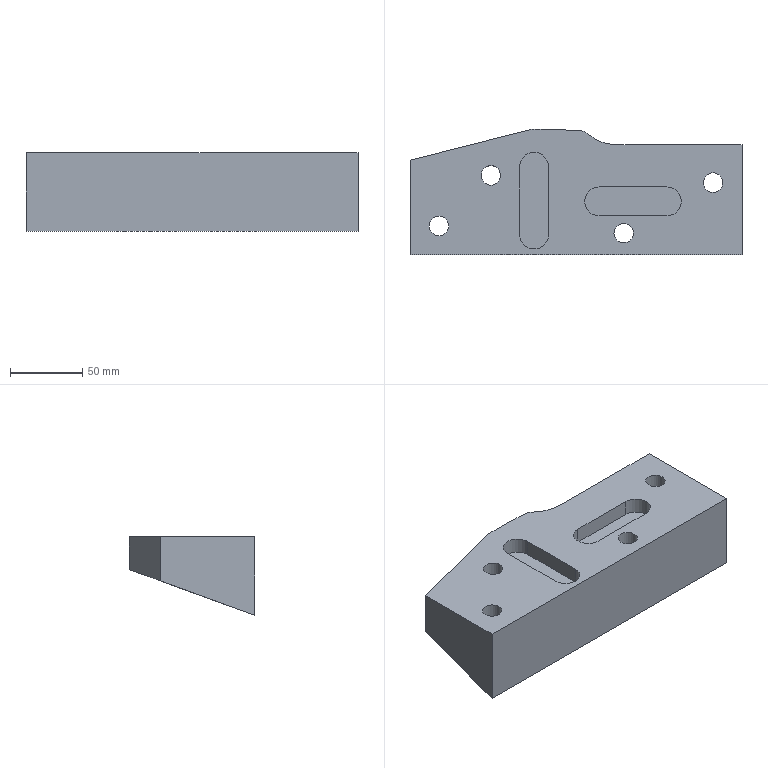Part | STEP file | lll_id3430_x_t | 1 solid | 44 faces | box 230 x 87.086 x 54.417 mm | volume 645334 mm3 | plane 20 | cylinder 18 | spline 4 | cone 2 | commonest cylinder face diameters 13.509 x4 20 x4 20.008 x4 10.505 x2 14 x2 19 x2
STEP:
#1=CARTESIAN_POINT('',(2625.,170.004,54.003));
#2=VERTEX_POINT('',#1);
#3=CARTESIAN_POINT('',(2625.,160.,50.362));
#4=DIRECTION('',(0.,-0.342,0.9397));
#5=DIRECTION('',(0.,0.9397,0.342));
#6=AXIS2_PLACEMENT_3D('',#3,#4,#5);
#7=ELLIPSE('',#6,10.646,10.004);
#8=EDGE_CURVE('',#2,#2,#7,.T.);
#9=ORIENTED_EDGE('',*,*,#8,.T.);
#10=EDGE_LOOP('',(#9));
#11=FACE_BOUND('',#10,.T.);
#12=CARTESIAN_POINT('',(2661.,205.004,66.742));
#13=VERTEX_POINT('',#12);
#14=CARTESIAN_POINT('',(2661.,195.,63.101));
#15=DIRECTION('',(0.,-0.342,0.9397));
#16=DIRECTION('',(0.,0.9397,0.342));
#17=AXIS2_PLACEMENT_3D('',#14,#15,#16);
#18=ELLIPSE('',#17,10.646,10.004);
#19=EDGE_CURVE('',#13,#13,#18,.T.);
#20=ORIENTED_EDGE('',*,*,#19,.T.);
#21=EDGE_LOOP('',(#20));
#22=FACE_BOUND('',#21,.T.);
#23=CARTESIAN_POINT('',(2650.,167.,52.91));
#24=VERTEX_POINT('',#23);
#25=CARTESIAN_POINT('',(2650.,160.,50.362));
#26=DIRECTION('',(0.,-0.342,0.9397));
#27=DIRECTION('',(0.,0.9397,0.342));
#28=AXIS2_PLACEMENT_3D('',#25,#26,#27);
#29=ELLIPSE('',#28,7.449,7.);
#30=EDGE_CURVE('',#24,#24,#29,.T.);
#31=ORIENTED_EDGE('',*,*,#30,.T.);
#32=EDGE_LOOP('',(#31));
#33=FACE_BOUND('',#32,.T.);
#34=CARTESIAN_POINT('',(2815.,200.004,64.922));
#35=VERTEX_POINT('',#34);
#36=CARTESIAN_POINT('',(2815.,190.,61.281));
#37=DIRECTION('',(0.,-0.342,0.9397));
#38=DIRECTION('',(0.,0.9397,0.342));
#39=AXIS2_PLACEMENT_3D('',#36,#37,#38);
#40=ELLIPSE('',#39,10.646,10.004);
#41=EDGE_CURVE('',#35,#35,#40,.T.);
#42=ORIENTED_EDGE('',*,*,#41,.T.);
#43=EDGE_LOOP('',(#42));
#44=FACE_BOUND('',#43,.T.);
#45=CARTESIAN_POINT('',(2753.,165.004,52.183));
#46=VERTEX_POINT('',#45);
#47=CARTESIAN_POINT('',(2753.,155.,48.542));
#48=DIRECTION('',(0.,-0.342,0.9397));
#49=DIRECTION('',(0.,0.9397,0.342));
#50=AXIS2_PLACEMENT_3D('',#47,#48,#49);
#51=ELLIPSE('',#50,10.646,10.004);
#52=EDGE_CURVE('',#46,#46,#51,.T.);
#53=ORIENTED_EDGE('',*,*,#52,.T.);
#54=EDGE_LOOP('',(#53));
#55=FACE_BOUND('',#54,.T.);
#56=CARTESIAN_POINT('',(2790.,167.,52.91));
#57=VERTEX_POINT('',#56);
#58=CARTESIAN_POINT('',(2790.,160.,50.362));
#59=DIRECTION('',(0.,-0.342,0.9397));
#60=DIRECTION('',(0.,0.9397,0.342));
#61=AXIS2_PLACEMENT_3D('',#58,#59,#60);
#62=ELLIPSE('',#61,7.449,7.);
#63=EDGE_CURVE('',#57,#57,#62,.T.);
#64=ORIENTED_EDGE('',*,*,#63,.T.);
#65=EDGE_LOOP('',(#64));
#66=FACE_BOUND('',#65,.T.);
#67=CARTESIAN_POINT('',(2835.,140.,43.083));
#68=VERTEX_POINT('',#67);
#69=CARTESIAN_POINT('',(2605.,140.,43.083));
#70=VERTEX_POINT('',#69);
#71=CARTESIAN_POINT('',(2720.,140.,43.083));
#72=DIRECTION('',(-1.,0.,0.));
#73=VECTOR('',#72,1.);
#74=LINE('',#71,#73);
#75=EDGE_CURVE('',#68,#70,#74,.T.);
#76=ORIENTED_EDGE('',*,*,#75,.T.);
#77=CARTESIAN_POINT('',(2605.,205.551,66.941));
#78=VERTEX_POINT('',#77);
#79=CARTESIAN_POINT('',(2605.,122.985,36.89));
#80=DIRECTION('',(0.,0.9397,0.342));
#81=VECTOR('',#80,1.);
#82=LINE('',#79,#81);
#83=EDGE_CURVE('',#70,#78,#82,.T.);
#84=ORIENTED_EDGE('',*,*,#83,.T.);
#85=CARTESIAN_POINT('',(2688.395,226.792,74.672));
#86=VERTEX_POINT('',#85);
#87=CARTESIAN_POINT('',(2701.697,230.18,75.905));
#88=DIRECTION('',(-0.9652,-0.2458,-0.08947));
#89=VECTOR('',#88,1.);
#90=LINE('',#87,#89);
#91=EDGE_CURVE('',#86,#78,#90,.T.);
#92=ORIENTED_EDGE('',*,*,#91,.F.);
#93=CARTESIAN_POINT('',(2691.864,227.019,74.755));
#94=VERTEX_POINT('',#93);
#95=CARTESIAN_POINT('',(2690.739,217.586,71.322));
#96=DIRECTION('',(0.,0.342,-0.9397));
#97=DIRECTION('',(0.,0.9397,0.342));
#98=AXIS2_PLACEMENT_3D('',#95,#96,#97);
#99=ELLIPSE('',#98,10.11,9.5);
#100=EDGE_CURVE('',#86,#94,#99,.T.);
#101=ORIENTED_EDGE('',*,*,#100,.T.);
#102=CARTESIAN_POINT('',(2695.813,226.8,74.675));
#103=VERTEX_POINT('',#102);
#104=CARTESIAN_POINT('',(2695.813,226.8,74.675));
#105=CARTESIAN_POINT('',(2695.461,226.798,74.675));
#106=CARTESIAN_POINT('',(2695.109,226.801,74.676));
#107=CARTESIAN_POINT('',(2694.758,226.81,74.679));
#108=CARTESIAN_POINT('',(2694.406,226.82,74.682));
#109=CARTESIAN_POINT('',(2694.054,226.834,74.688));
#110=CARTESIAN_POINT('',(2693.703,226.855,74.695));
#111=CARTESIAN_POINT('',(2693.089,226.892,74.709));
#112=CARTESIAN_POINT('',(2692.475,226.946,74.728));
#113=CARTESIAN_POINT('',(2691.864,227.019,74.755));
#114=B_SPLINE_CURVE_WITH_KNOTS('',3,(#104,#105,#106,#107,#108,#109,#110,#111,#112,#113),.UNSPECIFIED.,.F.,.F.,(4,3,3,4),(0.,0.2665,0.5331,1.),.UNSPECIFIED.);
#115=EDGE_CURVE('',#103,#94,#114,.T.);
#116=ORIENTED_EDGE('',*,*,#115,.F.);
#117=CARTESIAN_POINT('',(2704.997,226.806,74.677));
#118=VERTEX_POINT('',#117);
#119=CARTESIAN_POINT('',(2695.813,226.8,74.675));
#120=CARTESIAN_POINT('',(2696.59,226.825,74.685));
#121=CARTESIAN_POINT('',(2697.368,226.846,74.692));
#122=CARTESIAN_POINT('',(2698.146,226.859,74.697));
#123=CARTESIAN_POINT('',(2698.924,226.872,74.702));
#124=CARTESIAN_POINT('',(2699.703,226.879,74.704));
#125=CARTESIAN_POINT('',(2700.481,226.877,74.703));
#126=CARTESIAN_POINT('',(2701.986,226.873,74.702));
#127=CARTESIAN_POINT('',(2703.492,226.838,74.689));
#128=CARTESIAN_POINT('',(2704.997,226.806,74.677));
#129=B_SPLINE_CURVE_WITH_KNOTS('',3,(#119,#120,#121,#122,#123,#124,#125,#126,#127,#128),.UNSPECIFIED.,.F.,.F.,(4,3,3,4),(0.,0.2541,0.5082,1.),.UNSPECIFIED.);
#130=EDGE_CURVE('',#103,#118,#129,.T.);
#131=ORIENTED_EDGE('',*,*,#130,.T.);
#132=CARTESIAN_POINT('',(2722.606,226.048,74.402));
#133=VERTEX_POINT('',#132);
#134=CARTESIAN_POINT('',(2737.607,225.403,74.167));
#135=DIRECTION('',(-0.999,0.04298,0.01564));
#136=VECTOR('',#135,1.);
#137=LINE('',#134,#136);
#138=EDGE_CURVE('',#133,#118,#137,.T.);
#139=ORIENTED_EDGE('',*,*,#138,.F.);
#140=CARTESIAN_POINT('',(2728.715,223.469,73.463));
#141=VERTEX_POINT('',#140);
#142=CARTESIAN_POINT('',(2722.197,216.557,70.947));
#143=DIRECTION('',(0.,-0.342,0.9397));
#144=DIRECTION('',(0.,0.9397,0.342));
#145=AXIS2_PLACEMENT_3D('',#142,#143,#144);
#146=ELLIPSE('',#145,10.11,9.5);
#147=EDGE_CURVE('',#141,#133,#146,.T.);
#148=ORIENTED_EDGE('',*,*,#147,.F.);
#149=CARTESIAN_POINT('',(2744.457,216.509,70.93));
#150=VERTEX_POINT('',#149);
#151=CARTESIAN_POINT('',(2744.457,216.509,70.93));
#152=CARTESIAN_POINT('',(2738.528,217.02,71.115));
#153=CARTESIAN_POINT('',(2732.917,219.506,72.02));
#154=CARTESIAN_POINT('',(2728.715,223.469,73.463));
#155=B_SPLINE_CURVE_WITH_KNOTS('',3,(#151,#152,#153,#154),.UNSPECIFIED.,.F.,.F.,(4,4),(0.,1.),.UNSPECIFIED.);
#156=EDGE_CURVE('',#150,#141,#155,.T.);
#157=ORIENTED_EDGE('',*,*,#156,.F.);
#158=CARTESIAN_POINT('',(2753.979,216.1,70.781));
#159=VERTEX_POINT('',#158);
#160=CARTESIAN_POINT('',(2744.457,216.509,70.93));
#161=CARTESIAN_POINT('',(2745.266,216.439,70.904));
#162=CARTESIAN_POINT('',(2746.076,216.379,70.882));
#163=CARTESIAN_POINT('',(2746.887,216.327,70.863));
#164=CARTESIAN_POINT('',(2747.698,216.275,70.844));
#165=CARTESIAN_POINT('',(2748.509,216.232,70.829));
#166=CARTESIAN_POINT('',(2749.321,216.198,70.816));
#167=CARTESIAN_POINT('',(2750.873,216.133,70.793));
#168=CARTESIAN_POINT('',(2752.426,216.1,70.781));
#169=CARTESIAN_POINT('',(2753.979,216.1,70.781));
#170=B_SPLINE_CURVE_WITH_KNOTS('',3,(#160,#161,#162,#163,#164,#165,#166,#167,#168,#169),.UNSPECIFIED.,.F.,.F.,(4,3,3,4),(0.,0.2557,0.5114,1.),.UNSPECIFIED.);
#171=EDGE_CURVE('',#150,#159,#170,.T.);
#172=ORIENTED_EDGE('',*,*,#171,.T.);
#173=CARTESIAN_POINT('',(2835.,216.1,70.781));
#174=VERTEX_POINT('',#173);
#175=CARTESIAN_POINT('',(2732.617,216.1,70.781));
#176=DIRECTION('',(1.,0.,0.));
#177=VECTOR('',#176,1.);
#178=LINE('',#175,#177);
#179=EDGE_CURVE('',#159,#174,#178,.T.);
#180=ORIENTED_EDGE('',*,*,#179,.T.);
#181=CARTESIAN_POINT('',(2835.,62.167,14.754));
#182=DIRECTION('',(0.,0.9397,0.342));
#183=VECTOR('',#182,1.);
#184=LINE('',#181,#183);
#185=EDGE_CURVE('',#68,#174,#184,.T.);
#186=ORIENTED_EDGE('',*,*,#185,.F.);
#187=EDGE_LOOP('',(#76,#84,#92,#101,#116,#131,#139,#148,#157,#172,#180,#186));
#188=FACE_BOUND('',#187,.T.);
#189=CARTESIAN_POINT('',(2732.617,122.985,36.89));
#190=DIRECTION('',(0.,-0.342,0.9397));
#191=DIRECTION('',(0.,0.9397,0.342));
#192=AXIS2_PLACEMENT_3D('',#189,#190,#191);
#193=PLANE('',#192);
#194=ADVANCED_FACE('',(#11,#22,#33,#44,#55,#66,#188),#193,.F.);
#195=CARTESIAN_POINT('',(2783.,167.,97.5));
#196=VERTEX_POINT('',#195);
#197=CARTESIAN_POINT('',(2736.,167.,97.5));
#198=VERTEX_POINT('',#197);
#199=CARTESIAN_POINT('',(2685.,167.,97.5));
#200=DIRECTION('',(-1.,0.,0.));
#201=VECTOR('',#200,1.);
#202=LINE('',#199,#201);
#203=EDGE_CURVE('',#196,#198,#202,.T.);
#204=ORIENTED_EDGE('',*,*,#203,.T.);
#205=CARTESIAN_POINT('',(2736.,187.,97.5));
#206=VERTEX_POINT('',#205);
#207=CARTESIAN_POINT('',(2736.,177.,97.5));
#208=DIRECTION('',(0.,0.,-1.));
#209=DIRECTION('',(-1.,0.,0.));
#210=AXIS2_PLACEMENT_3D('',#207,#208,#209);
#211=CIRCLE('',#210,10.);
#212=EDGE_CURVE('',#198,#206,#211,.T.);
#213=ORIENTED_EDGE('',*,*,#212,.T.);
#214=CARTESIAN_POINT('',(2783.,187.,97.5));
#215=VERTEX_POINT('',#214);
#216=CARTESIAN_POINT('',(2685.,187.,97.5));
#217=DIRECTION('',(1.,0.,0.));
#218=VECTOR('',#217,1.);
#219=LINE('',#216,#218);
#220=EDGE_CURVE('',#206,#215,#219,.T.);
#221=ORIENTED_EDGE('',*,*,#220,.T.);
#222=CARTESIAN_POINT('',(2783.,177.,97.5));
#223=DIRECTION('',(0.,0.,-1.));
#224=DIRECTION('',(-1.,0.,0.));
#225=AXIS2_PLACEMENT_3D('',#222,#223,#224);
#226=CIRCLE('',#225,10.);
#227=EDGE_CURVE('',#215,#196,#226,.T.);
#228=ORIENTED_EDGE('',*,*,#227,.T.);
#229=EDGE_LOOP('',(#204,#213,#221,#228));
#230=FACE_BOUND('',#229,.T.);
#231=CARTESIAN_POINT('',(2701.,201.,97.5));
#232=VERTEX_POINT('',#231);
#233=CARTESIAN_POINT('',(2701.,154.,97.5));
#234=VERTEX_POINT('',#233);
#235=CARTESIAN_POINT('',(2701.,0.00007422,97.5));
#236=DIRECTION('',(0.,-1.,0.));
#237=VECTOR('',#236,1.);
#238=LINE('',#235,#237);
#239=EDGE_CURVE('',#232,#234,#238,.T.);
#240=ORIENTED_EDGE('',*,*,#239,.T.);
#241=CARTESIAN_POINT('',(2681.,154.,97.5));
#242=VERTEX_POINT('',#241);
#243=CARTESIAN_POINT('',(2691.,154.,97.5));
#244=DIRECTION('',(0.,0.,-1.));
#245=DIRECTION('',(-1.,0.,0.));
#246=AXIS2_PLACEMENT_3D('',#243,#244,#245);
#247=CIRCLE('',#246,10.);
#248=EDGE_CURVE('',#234,#242,#247,.T.);
#249=ORIENTED_EDGE('',*,*,#248,.T.);
#250=CARTESIAN_POINT('',(2681.,201.,97.5));
#251=VERTEX_POINT('',#250);
#252=CARTESIAN_POINT('',(2681.,0.00007422,97.5));
#253=DIRECTION('',(0.,1.,0.));
#254=VECTOR('',#253,1.);
#255=LINE('',#252,#254);
#256=EDGE_CURVE('',#242,#251,#255,.T.);
#257=ORIENTED_EDGE('',*,*,#256,.T.);
#258=CARTESIAN_POINT('',(2691.,201.,97.5));
#259=DIRECTION('',(0.,0.,-1.));
#260=DIRECTION('',(-1.,0.,0.));
#261=AXIS2_PLACEMENT_3D('',#258,#259,#260);
#262=CIRCLE('',#261,10.);
#263=EDGE_CURVE('',#251,#232,#262,.T.);
#264=ORIENTED_EDGE('',*,*,#263,.T.);
#265=EDGE_LOOP('',(#240,#249,#257,#264));
#266=FACE_BOUND('',#265,.T.);
#267=CARTESIAN_POINT('',(2618.245,160.,97.5));
#268=VERTEX_POINT('',#267);
#269=CARTESIAN_POINT('',(2625.,160.,97.5));
#270=DIRECTION('',(0.,0.,-1.));
#271=DIRECTION('',(-1.,0.,0.));
#272=AXIS2_PLACEMENT_3D('',#269,#270,#271);
#273=CIRCLE('',#272,6.755);
#274=EDGE_CURVE('',#268,#268,#273,.T.);
#275=ORIENTED_EDGE('',*,*,#274,.T.);
#276=EDGE_LOOP('',(#275));
#277=FACE_BOUND('',#276,.T.);
#278=CARTESIAN_POINT('',(2654.245,195.,97.5));
#279=VERTEX_POINT('',#278);
#280=CARTESIAN_POINT('',(2661.,195.,97.5));
#281=DIRECTION('',(0.,0.,-1.));
#282=DIRECTION('',(-1.,0.,0.));
#283=AXIS2_PLACEMENT_3D('',#280,#281,#282);
#284=CIRCLE('',#283,6.755);
#285=EDGE_CURVE('',#279,#279,#284,.T.);
#286=ORIENTED_EDGE('',*,*,#285,.T.);
#287=EDGE_LOOP('',(#286));
#288=FACE_BOUND('',#287,.T.);
#289=CARTESIAN_POINT('',(2808.245,190.,97.5));
#290=VERTEX_POINT('',#289);
#291=CARTESIAN_POINT('',(2815.,190.,97.5));
#292=DIRECTION('',(0.,0.,-1.));
#293=DIRECTION('',(-1.,0.,0.));
#294=AXIS2_PLACEMENT_3D('',#291,#292,#293);
#295=CIRCLE('',#294,6.755);
#296=EDGE_CURVE('',#290,#290,#295,.T.);
#297=ORIENTED_EDGE('',*,*,#296,.T.);
#298=EDGE_LOOP('',(#297));
#299=FACE_BOUND('',#298,.T.);
#300=CARTESIAN_POINT('',(2746.245,155.,97.5));
#301=VERTEX_POINT('',#300);
#302=CARTESIAN_POINT('',(2753.,155.,97.5));
#303=DIRECTION('',(0.,0.,-1.));
#304=DIRECTION('',(-1.,0.,0.));
#305=AXIS2_PLACEMENT_3D('',#302,#303,#304);
#306=CIRCLE('',#305,6.755);
#307=EDGE_CURVE('',#301,#301,#306,.T.);
#308=ORIENTED_EDGE('',*,*,#307,.T.);
#309=EDGE_LOOP('',(#308));
#310=FACE_BOUND('',#309,.T.);
#311=CARTESIAN_POINT('',(2835.,140.,97.5));
#312=VERTEX_POINT('',#311);
#313=CARTESIAN_POINT('',(2605.,140.,97.5));
#314=VERTEX_POINT('',#313);
#315=CARTESIAN_POINT('',(2685.,140.,97.5));
#316=DIRECTION('',(-1.,0.,0.));
#317=VECTOR('',#316,1.);
#318=LINE('',#315,#317);
#319=EDGE_CURVE('',#312,#314,#318,.T.);
#320=ORIENTED_EDGE('',*,*,#319,.F.);
#321=CARTESIAN_POINT('',(2835.,216.1,97.5));
#322=VERTEX_POINT('',#321);
#323=CARTESIAN_POINT('',(2835.,0.00007422,97.5));
#324=DIRECTION('',(0.,1.,0.));
#325=VECTOR('',#324,1.);
#326=LINE('',#323,#325);
#327=EDGE_CURVE('',#312,#322,#326,.T.);
#328=ORIENTED_EDGE('',*,*,#327,.T.);
#329=CARTESIAN_POINT('',(2753.979,216.1,97.5));
#330=VERTEX_POINT('',#329);
#331=CARTESIAN_POINT('',(2753.979,216.1,97.5));
#332=DIRECTION('',(1.,0.,0.));
#333=VECTOR('',#332,1.);
#334=LINE('',#331,#333);
#335=EDGE_CURVE('',#330,#322,#334,.T.);
#336=ORIENTED_EDGE('',*,*,#335,.F.);
#337=CARTESIAN_POINT('',(2744.457,216.509,97.5));
#338=VERTEX_POINT('',#337);
#339=CARTESIAN_POINT('',(2753.979,216.1,97.5));
#340=CARTESIAN_POINT('',(2753.166,216.1,97.5));
#341=CARTESIAN_POINT('',(2752.353,216.109,97.5));
#342=CARTESIAN_POINT('',(2751.541,216.127,97.5));
#343=CARTESIAN_POINT('',(2750.728,216.145,97.5));
#344=CARTESIAN_POINT('',(2749.916,216.171,97.5));
#345=CARTESIAN_POINT('',(2749.104,216.207,97.5));
#346=CARTESIAN_POINT('',(2747.553,216.275,97.5));
#347=CARTESIAN_POINT('',(2746.003,216.376,97.5));
#348=CARTESIAN_POINT('',(2744.457,216.509,97.5));
#349=B_SPLINE_CURVE_WITH_KNOTS('',3,(#339,#340,#341,#342,#343,#344,#345,#346,#347,#348),.UNSPECIFIED.,.F.,.F.,(4,3,3,4),(0.,0.2557,0.5115,1.),.UNSPECIFIED.);
#350=EDGE_CURVE('',#330,#338,#349,.T.);
#351=ORIENTED_EDGE('',*,*,#350,.T.);
#352=CARTESIAN_POINT('',(2728.715,223.469,97.5));
#353=VERTEX_POINT('',#352);
#354=CARTESIAN_POINT('',(2728.715,223.469,97.5));
#355=CARTESIAN_POINT('',(2732.994,219.433,97.5));
#356=CARTESIAN_POINT('',(2738.6,217.013,97.5));
#357=CARTESIAN_POINT('',(2744.457,216.509,97.5));
#358=B_SPLINE_CURVE_WITH_KNOTS('',3,(#354,#355,#356,#357),.UNSPECIFIED.,.F.,.F.,(4,4),(0.,1.),.UNSPECIFIED.);
#359=EDGE_CURVE('',#353,#338,#358,.T.);
#360=ORIENTED_EDGE('',*,*,#359,.F.);
#361=CARTESIAN_POINT('',(2722.606,226.048,97.5));
#362=VERTEX_POINT('',#361);
#363=CARTESIAN_POINT('',(2722.197,216.557,97.5));
#364=DIRECTION('',(0.,0.,1.));
#365=DIRECTION('',(-1.,0.,0.));
#366=AXIS2_PLACEMENT_3D('',#363,#364,#365);
#367=CIRCLE('',#366,9.5);
#368=EDGE_CURVE('',#353,#362,#367,.T.);
#369=ORIENTED_EDGE('',*,*,#368,.T.);
#370=CARTESIAN_POINT('',(2704.997,226.806,97.5));
#371=VERTEX_POINT('',#370);
#372=CARTESIAN_POINT('',(2694.776,227.245,97.5));
#373=DIRECTION('',(0.9991,-0.04298,0.));
#374=VECTOR('',#373,1.);
#375=LINE('',#372,#374);
#376=EDGE_CURVE('',#371,#362,#375,.T.);
#377=ORIENTED_EDGE('',*,*,#376,.F.);
#378=CARTESIAN_POINT('',(2695.813,226.8,97.5));
#379=VERTEX_POINT('',#378);
#380=CARTESIAN_POINT('',(2695.813,226.8,97.5));
#381=CARTESIAN_POINT('',(2696.59,226.825,97.5));
#382=CARTESIAN_POINT('',(2697.368,226.846,97.5));
#383=CARTESIAN_POINT('',(2698.146,226.859,97.5));
#384=CARTESIAN_POINT('',(2698.924,226.872,97.5));
#385=CARTESIAN_POINT('',(2699.703,226.879,97.5));
#386=CARTESIAN_POINT('',(2700.481,226.877,97.5));
#387=CARTESIAN_POINT('',(2701.987,226.873,97.5));
#388=CARTESIAN_POINT('',(2703.492,226.838,97.5));
#389=CARTESIAN_POINT('',(2704.997,226.806,97.5));
#390=B_SPLINE_CURVE_WITH_KNOTS('',3,(#380,#381,#382,#383,#384,#385,#386,#387,#388,#389),.UNSPECIFIED.,.F.,.F.,(4,3,3,4),(0.,0.2541,0.5082,1.),.UNSPECIFIED.);
#391=EDGE_CURVE('',#379,#371,#390,.T.);
#392=ORIENTED_EDGE('',*,*,#391,.F.);
#393=CARTESIAN_POINT('',(2691.864,227.019,97.5));
#394=VERTEX_POINT('',#393);
#395=CARTESIAN_POINT('',(2695.813,226.8,97.5));
#396=CARTESIAN_POINT('',(2695.461,226.798,97.5));
#397=CARTESIAN_POINT('',(2695.109,226.801,97.5));
#398=CARTESIAN_POINT('',(2694.758,226.81,97.5));
#399=CARTESIAN_POINT('',(2694.406,226.82,97.5));
#400=CARTESIAN_POINT('',(2694.054,226.834,97.5));
#401=CARTESIAN_POINT('',(2693.703,226.855,97.5));
#402=CARTESIAN_POINT('',(2693.089,226.892,97.5));
#403=CARTESIAN_POINT('',(2692.475,226.946,97.5));
#404=CARTESIAN_POINT('',(2691.864,227.019,97.5));
#405=B_SPLINE_CURVE_WITH_KNOTS('',3,(#395,#396,#397,#398,#399,#400,#401,#402,#403,#404),.UNSPECIFIED.,.F.,.F.,(4,3,3,4),(0.,0.2666,0.5332,1.),.UNSPECIFIED.);
#406=EDGE_CURVE('',#379,#394,#405,.T.);
#407=ORIENTED_EDGE('',*,*,#406,.T.);
#408=CARTESIAN_POINT('',(2688.395,226.792,97.5));
#409=VERTEX_POINT('',#408);
#410=CARTESIAN_POINT('',(2690.739,217.586,97.5));
#411=DIRECTION('',(0.,0.,-1.));
#412=DIRECTION('',(-1.,0.,0.));
#413=AXIS2_PLACEMENT_3D('',#410,#411,#412);
#414=CIRCLE('',#413,9.5);
#415=EDGE_CURVE('',#409,#394,#414,.T.);
#416=ORIENTED_EDGE('',*,*,#415,.F.);
#417=CARTESIAN_POINT('',(2605.,205.551,97.5));
#418=VERTEX_POINT('',#417);
#419=CARTESIAN_POINT('',(2630.962,212.164,97.5));
#420=DIRECTION('',(0.9691,0.2468,0.));
#421=VECTOR('',#420,1.);
#422=LINE('',#419,#421);
#423=EDGE_CURVE('',#418,#409,#422,.T.);
#424=ORIENTED_EDGE('',*,*,#423,.F.);
#425=CARTESIAN_POINT('',(2605.,0.,97.5));
#426=DIRECTION('',(0.,-1.,0.));
#427=VECTOR('',#426,1.);
#428=LINE('',#425,#427);
#429=EDGE_CURVE('',#418,#314,#428,.T.);
#430=ORIENTED_EDGE('',*,*,#429,.T.);
#431=EDGE_LOOP('',(#320,#328,#336,#351,#360,#369,#377,#392,#407,#416,#424,#430));
#432=FACE_BOUND('',#431,.T.);
#433=CARTESIAN_POINT('',(2685.,0.00007422,97.5));
#434=DIRECTION('',(0.,0.,-1.));
#435=DIRECTION('',(1.,0.,0.));
#436=AXIS2_PLACEMENT_3D('',#433,#434,#435);
#437=PLANE('',#436);
#438=ADVANCED_FACE('',(#230,#266,#277,#288,#299,#310,#432),#437,.F.);
#439=CARTESIAN_POINT('',(2835.,140.,652.5));
#440=DIRECTION('',(0.,0.,1.));
#441=VECTOR('',#440,1.);
#442=LINE('',#439,#441);
#443=EDGE_CURVE('',#68,#312,#442,.T.);
#444=ORIENTED_EDGE('',*,*,#443,.F.);
#445=ORIENTED_EDGE('',*,*,#185,.T.);
#446=CARTESIAN_POINT('',(2835.,216.1,652.5));
#447=DIRECTION('',(0.,0.,1.));
#448=VECTOR('',#447,1.);
#449=LINE('',#446,#448);
#450=EDGE_CURVE('',#174,#322,#449,.T.);
#451=ORIENTED_EDGE('',*,*,#450,.T.);
#452=ORIENTED_EDGE('',*,*,#327,.F.);
#453=EDGE_LOOP('',(#444,#445,#451,#452));
#454=FACE_OUTER_BOUND('',#453,.T.);
#455=CARTESIAN_POINT('',(2835.,-169.953,652.5));
#456=DIRECTION('',(-1.,0.,0.));
#457=DIRECTION('',(0.,0.,-1.));
#458=AXIS2_PLACEMENT_3D('',#455,#456,#457);
#459=PLANE('',#458);
#460=ADVANCED_FACE('',(#454),#459,.F.);
#461=ORIENTED_EDGE('',*,*,#83,.F.);
#462=CARTESIAN_POINT('',(2605.,140.,52.5));
#463=DIRECTION('',(0.,0.,-1.));
#464=VECTOR('',#463,1.);
#465=LINE('',#462,#464);
#466=EDGE_CURVE('',#314,#70,#465,.T.);
#467=ORIENTED_EDGE('',*,*,#466,.F.);
#468=ORIENTED_EDGE('',*,*,#429,.F.);
#469=CARTESIAN_POINT('',(2605.,205.551,-74.226));
#470=DIRECTION('',(0.,0.,-1.));
#471=VECTOR('',#470,1.);
#472=LINE('',#469,#471);
#473=EDGE_CURVE('',#418,#78,#472,.T.);
#474=ORIENTED_EDGE('',*,*,#473,.T.);
#475=EDGE_LOOP('',(#461,#467,#468,#474));
#476=FACE_OUTER_BOUND('',#475,.T.);
#477=CARTESIAN_POINT('',(2605.,0.,52.5));
#478=DIRECTION('',(-1.,0.,0.));
#479=DIRECTION('',(0.,0.,1.));
#480=AXIS2_PLACEMENT_3D('',#477,#478,#479);
#481=PLANE('',#480);
#482=ADVANCED_FACE('',(#476),#481,.T.);
#483=ORIENTED_EDGE('',*,*,#91,.T.);
#484=ORIENTED_EDGE('',*,*,#473,.F.);
#485=ORIENTED_EDGE('',*,*,#423,.T.);
#486=CARTESIAN_POINT('',(2688.395,226.792,-74.226));
#487=DIRECTION('',(0.,0.,-1.));
#488=VECTOR('',#487,1.);
#489=LINE('',#486,#488);
#490=EDGE_CURVE('',#409,#86,#489,.T.);
#491=ORIENTED_EDGE('',*,*,#490,.T.);
#492=EDGE_LOOP('',(#483,#484,#485,#491));
#493=FACE_OUTER_BOUND('',#492,.T.);
#494=CARTESIAN_POINT('',(2690.762,227.395,-74.226));
#495=DIRECTION('',(-0.2468,0.9691,0.));
#496=DIRECTION('',(-0.9691,-0.2468,0.));
#497=AXIS2_PLACEMENT_3D('',#494,#495,#496);
#498=PLANE('',#497);
#499=ADVANCED_FACE('',(#493),#498,.T.);
#500=ORIENTED_EDGE('',*,*,#415,.T.);
#501=CARTESIAN_POINT('',(2691.864,227.019,-74.342));
#502=DIRECTION('',(0.,0.,1.));
#503=VECTOR('',#502,1.);
#504=LINE('',#501,#503);
#505=EDGE_CURVE('',#94,#394,#504,.T.);
#506=ORIENTED_EDGE('',*,*,#505,.F.);
#507=ORIENTED_EDGE('',*,*,#100,.F.);
#508=ORIENTED_EDGE('',*,*,#490,.F.);
#509=EDGE_LOOP('',(#500,#506,#507,#508));
#510=FACE_OUTER_BOUND('',#509,.T.);
#511=CARTESIAN_POINT('',(2690.739,217.586,75.739));
#512=DIRECTION('',(0.,0.,1.));
#513=DIRECTION('',(-1.,0.,0.));
#514=AXIS2_PLACEMENT_3D('',#511,#512,#513);
#515=CYLINDRICAL_SURFACE('',#514,9.5);
#516=ADVANCED_FACE('',(#510),#515,.T.);
#517=ORIENTED_EDGE('',*,*,#406,.F.);
#518=CARTESIAN_POINT('',(2695.813,226.8,74.675));
#519=DIRECTION('',(0.,0.,1.));
#520=VECTOR('',#519,1.);
#521=LINE('',#518,#520);
#522=EDGE_CURVE('',#103,#379,#521,.T.);
#523=ORIENTED_EDGE('',*,*,#522,.F.);
#524=ORIENTED_EDGE('',*,*,#115,.T.);
#525=ORIENTED_EDGE('',*,*,#505,.T.);
#526=EDGE_LOOP('',(#517,#523,#524,#525));
#527=FACE_OUTER_BOUND('',#526,.T.);
#528=CARTESIAN_POINT('',(2695.813,226.8,74.538));
#529=CARTESIAN_POINT('',(2695.813,226.8,97.638));
#530=CARTESIAN_POINT('',(2695.509,226.798,74.538));
#531=CARTESIAN_POINT('',(2695.509,226.798,97.637));
#532=CARTESIAN_POINT('',(2695.157,226.801,74.538));
#533=CARTESIAN_POINT('',(2695.157,226.801,97.638));
#534=CARTESIAN_POINT('',(2694.498,226.816,74.544));
#535=CARTESIAN_POINT('',(2694.498,226.816,97.644));
#536=CARTESIAN_POINT('',(2693.509,226.855,74.557));
#537=CARTESIAN_POINT('',(2693.509,226.855,97.657));
#538=CARTESIAN_POINT('',(2692.521,226.941,74.585));
#539=CARTESIAN_POINT('',(2692.521,226.941,97.685));
#540=CARTESIAN_POINT('',(2691.864,227.019,74.612));
#541=CARTESIAN_POINT('',(2691.864,227.019,97.711));
#542=B_SPLINE_SURFACE_WITH_KNOTS('',3,1,((#528,#529),(#530,#531),(#532,#533),(#534,#535),(#536,#537),(#538,#539),(#540,#541)),.UNSPECIFIED.,.F.,.F.,.F.,(4,2,1,4),(2,2),(0.,0.25,0.5,1.),(0.,1.),.UNSPECIFIED.);
#543=ADVANCED_FACE('',(#527),#542,.T.);
#544=ORIENTED_EDGE('',*,*,#391,.T.);
#545=CARTESIAN_POINT('',(2704.997,226.806,74.677));
#546=DIRECTION('',(0.,0.,1.));
#547=VECTOR('',#546,1.);
#548=LINE('',#545,#547);
#549=EDGE_CURVE('',#118,#371,#548,.T.);
#550=ORIENTED_EDGE('',*,*,#549,.F.);
#551=ORIENTED_EDGE('',*,*,#130,.F.);
#552=ORIENTED_EDGE('',*,*,#522,.T.);
#553=EDGE_LOOP('',(#544,#550,#551,#552));
#554=FACE_OUTER_BOUND('',#553,.T.);
#555=CARTESIAN_POINT('',(2704.997,226.806,74.54));
#556=CARTESIAN_POINT('',(2704.997,226.806,97.639));
#557=CARTESIAN_POINT('',(2703.442,226.839,74.552));
#558=CARTESIAN_POINT('',(2703.442,226.839,97.652));
#559=CARTESIAN_POINT('',(2701.905,226.874,74.565));
#560=CARTESIAN_POINT('',(2701.905,226.874,97.664));
#561=CARTESIAN_POINT('',(2698.867,226.879,74.567));
#562=CARTESIAN_POINT('',(2698.867,226.879,97.666));
#563=CARTESIAN_POINT('',(2697.365,226.851,74.556));
#564=CARTESIAN_POINT('',(2697.365,226.851,97.656));
#565=CARTESIAN_POINT('',(2695.813,226.8,74.538));
#566=CARTESIAN_POINT('',(2695.813,226.8,97.637));
#567=B_SPLINE_SURFACE_WITH_KNOTS('',3,1,((#555,#556),(#557,#558),(#559,#560),(#561,#562),(#563,#564),(#565,#566)),.UNSPECIFIED.,.F.,.F.,.F.,(4,2,4),(2,2),(0.,0.5,1.),(0.,1.),.UNSPECIFIED.);
#568=ADVANCED_FACE('',(#554),#567,.T.);
#569=ORIENTED_EDGE('',*,*,#376,.T.);
#570=CARTESIAN_POINT('',(2722.606,226.048,-74.752));
#571=DIRECTION('',(0.,0.,-1.));
#572=VECTOR('',#571,1.);
#573=LINE('',#570,#572);
#574=EDGE_CURVE('',#362,#133,#573,.T.);
#575=ORIENTED_EDGE('',*,*,#574,.T.);
#576=ORIENTED_EDGE('',*,*,#138,.T.);
#577=ORIENTED_EDGE('',*,*,#549,.T.);
#578=EDGE_LOOP('',(#569,#575,#576,#577));
#579=FACE_OUTER_BOUND('',#578,.T.);
#580=CARTESIAN_POINT('',(2726.627,225.875,-74.752));
#581=DIRECTION('',(0.04298,0.9991,0.));
#582=DIRECTION('',(-0.9991,0.04298,0.));
#583=AXIS2_PLACEMENT_3D('',#580,#581,#582);
#584=PLANE('',#583);
#585=ADVANCED_FACE('',(#579),#584,.T.);
#586=ORIENTED_EDGE('',*,*,#368,.F.);
#587=CARTESIAN_POINT('',(2728.715,223.469,-75.875));
#588=DIRECTION('',(0.,0.,1.));
#589=VECTOR('',#588,1.);
#590=LINE('',#587,#589);
#591=EDGE_CURVE('',#141,#353,#590,.T.);
#592=ORIENTED_EDGE('',*,*,#591,.F.);
#593=ORIENTED_EDGE('',*,*,#147,.T.);
#594=ORIENTED_EDGE('',*,*,#574,.F.);
#595=EDGE_LOOP('',(#586,#592,#593,#594));
#596=FACE_OUTER_BOUND('',#595,.T.);
#597=CARTESIAN_POINT('',(2722.197,216.557,75.109));
#598=DIRECTION('',(0.,0.,1.));
#599=DIRECTION('',(-1.,0.,0.));
#600=AXIS2_PLACEMENT_3D('',#597,#598,#599);
#601=CYLINDRICAL_SURFACE('',#600,9.5);
#602=ADVANCED_FACE('',(#596),#601,.T.);
#603=ORIENTED_EDGE('',*,*,#591,.T.);
#604=ORIENTED_EDGE('',*,*,#359,.T.);
#605=CARTESIAN_POINT('',(2744.457,216.509,97.5));
#606=CARTESIAN_POINT('',(2744.457,216.509,88.643));
#607=CARTESIAN_POINT('',(2744.457,216.509,79.786));
#608=CARTESIAN_POINT('',(2744.457,216.509,70.93));
#609=B_SPLINE_CURVE_WITH_KNOTS('',3,(#605,#606,#607,#608),.UNSPECIFIED.,.F.,.F.,(4,4),(0.,1.),.UNSPECIFIED.);
#610=EDGE_CURVE('',#338,#150,#609,.T.);
#611=ORIENTED_EDGE('',*,*,#610,.T.);
#612=ORIENTED_EDGE('',*,*,#156,.T.);
#613=EDGE_LOOP('',(#603,#604,#611,#612));
#614=FACE_OUTER_BOUND('',#613,.T.);
#615=CARTESIAN_POINT('',(2744.457,216.509,70.77));
#616=CARTESIAN_POINT('',(2744.457,216.509,97.659));
#617=CARTESIAN_POINT('',(2744.29,216.523,70.775));
#618=CARTESIAN_POINT('',(2744.29,216.523,97.665));
#619=CARTESIAN_POINT('',(2744.089,216.543,70.781));
#620=CARTESIAN_POINT('',(2744.089,216.543,97.67));
#621=CARTESIAN_POINT('',(2743.723,216.582,70.794));
#622=CARTESIAN_POINT('',(2743.723,216.582,97.683));
#623=CARTESIAN_POINT('',(2743.174,216.646,70.816));
#624=CARTESIAN_POINT('',(2743.174,216.646,97.705));
#625=CARTESIAN_POINT('',(2742.627,216.728,70.842));
#626=CARTESIAN_POINT('',(2742.627,216.728,97.732));
#627=CARTESIAN_POINT('',(2741.539,216.912,70.903));
#628=CARTESIAN_POINT('',(2741.539,216.912,97.793));
#629=CARTESIAN_POINT('',(2740.819,217.065,70.954));
#630=CARTESIAN_POINT('',(2740.819,217.065,97.843));
#631=CARTESIAN_POINT('',(2738.684,217.61,71.134));
#632=CARTESIAN_POINT('',(2738.684,217.61,98.023));
#633=CARTESIAN_POINT('',(2737.293,218.089,71.292));
#634=CARTESIAN_POINT('',(2737.293,218.089,98.181));
#635=CARTESIAN_POINT('',(2733.275,219.859,71.875));
#636=CARTESIAN_POINT('',(2733.275,219.859,98.764));
#637=CARTESIAN_POINT('',(2730.814,221.489,72.41));
#638=CARTESIAN_POINT('',(2730.814,221.489,99.3));
#639=CARTESIAN_POINT('',(2728.715,223.469,73.059));
#640=CARTESIAN_POINT('',(2728.715,223.469,99.948));
#641=B_SPLINE_SURFACE_WITH_KNOTS('',3,1,((#615,#616),(#617,#618),(#619,#620),(#621,#622),(#623,#624),(#625,#626),(#627,#628),(#629,#630),(#631,#632),(#633,#634),(#635,#636),(#637,#638),(#639,#640)),.UNSPECIFIED.,.F.,.F.,.F.,(4,2,1,2,2,2,4),(2,2),(0.,0.03125,0.0625,0.125,0.25,0.5,1.),(0.,1.),.UNSPECIFIED.);
#642=ADVANCED_FACE('',(#614),#641,.T.);
#643=ORIENTED_EDGE('',*,*,#610,.F.);
#644=ORIENTED_EDGE('',*,*,#350,.F.);
#645=CARTESIAN_POINT('',(2753.979,216.1,-78.309));
#646=DIRECTION('',(0.,0.,-1.));
#647=VECTOR('',#646,1.);
#648=LINE('',#645,#647);
#649=EDGE_CURVE('',#330,#159,#648,.T.);
#650=ORIENTED_EDGE('',*,*,#649,.T.);
#651=ORIENTED_EDGE('',*,*,#171,.F.);
#652=EDGE_LOOP('',(#643,#644,#650,#651));
#653=FACE_OUTER_BOUND('',#652,.T.);
#654=CARTESIAN_POINT('',(2753.979,216.1,70.62));
#655=CARTESIAN_POINT('',(2753.979,216.1,97.66));
#656=CARTESIAN_POINT('',(2752.389,216.1,70.62));
#657=CARTESIAN_POINT('',(2752.389,216.1,97.66));
#658=CARTESIAN_POINT('',(2750.006,216.151,70.639));
#659=CARTESIAN_POINT('',(2750.006,216.151,97.679));
#660=CARTESIAN_POINT('',(2747.626,216.279,70.684));
#661=CARTESIAN_POINT('',(2747.626,216.279,97.724));
#662=CARTESIAN_POINT('',(2746.041,216.381,70.721));
#663=CARTESIAN_POINT('',(2746.041,216.381,97.76));
#664=CARTESIAN_POINT('',(2745.231,216.442,70.742));
#665=CARTESIAN_POINT('',(2745.231,216.442,97.782));
#666=CARTESIAN_POINT('',(2744.457,216.509,70.766));
#667=CARTESIAN_POINT('',(2744.457,216.509,97.806));
#668=B_SPLINE_SURFACE_WITH_KNOTS('',3,1,((#654,#655),(#656,#657),(#658,#659),(#660,#661),(#662,#663),(#664,#665),(#666,#667)),.UNSPECIFIED.,.F.,.F.,.F.,(4,1,2,4),(2,2),(0.,0.5,0.75,1.),(0.,1.),.UNSPECIFIED.);
#669=ADVANCED_FACE('',(#653),#668,.T.);
#670=ORIENTED_EDGE('',*,*,#649,.F.);
#671=ORIENTED_EDGE('',*,*,#335,.T.);
#672=ORIENTED_EDGE('',*,*,#450,.F.);
#673=ORIENTED_EDGE('',*,*,#179,.F.);
#674=EDGE_LOOP('',(#670,#671,#672,#673));
#675=FACE_OUTER_BOUND('',#674,.T.);
#676=CARTESIAN_POINT('',(2753.979,216.1,-78.309));
#677=DIRECTION('',(0.,-1.,0.));
#678=DIRECTION('',(1.,0.,0.));
#679=AXIS2_PLACEMENT_3D('',#676,#677,#678);
#680=PLANE('',#679);
#681=ADVANCED_FACE('',(#675),#680,.F.);
#682=ORIENTED_EDGE('',*,*,#75,.F.);
#683=ORIENTED_EDGE('',*,*,#443,.T.);
#684=ORIENTED_EDGE('',*,*,#319,.T.);
#685=ORIENTED_EDGE('',*,*,#466,.T.);
#686=EDGE_LOOP('',(#682,#683,#684,#685));
#687=FACE_OUTER_BOUND('',#686,.T.);
#688=CARTESIAN_POINT('',(2720.,140.,52.5));
#689=DIRECTION('',(0.,-1.,0.));
#690=DIRECTION('',(0.,0.,-1.));
#691=AXIS2_PLACEMENT_3D('',#688,#689,#690);
#692=PLANE('',#691);
#693=ADVANCED_FACE('',(#687),#692,.T.);
#694=CARTESIAN_POINT('',(2797.,160.,57.5));
#695=VERTEX_POINT('',#694);
#696=CARTESIAN_POINT('',(2790.,160.,57.5));
#697=DIRECTION('',(0.,0.,1.));
#698=DIRECTION('',(1.,0.,0.));
#699=AXIS2_PLACEMENT_3D('',#696,#697,#698);
#700=CIRCLE('',#699,7.);
#701=EDGE_CURVE('',#695,#695,#700,.T.);
#702=ORIENTED_EDGE('',*,*,#701,.T.);
#703=EDGE_LOOP('',(#702));
#704=FACE_BOUND('',#703,.T.);
#705=ORIENTED_EDGE('',*,*,#63,.F.);
#706=EDGE_LOOP('',(#705));
#707=FACE_BOUND('',#706,.T.);
#708=CARTESIAN_POINT('',(2790.,160.,42.5));
#709=DIRECTION('',(0.,0.,1.));
#710=DIRECTION('',(1.,0.,0.));
#711=AXIS2_PLACEMENT_3D('',#708,#709,#710);
#712=CYLINDRICAL_SURFACE('',#711,7.);
#713=ADVANCED_FACE('',(#704,#707),#712,.F.);
#714=CARTESIAN_POINT('',(2795.253,160.,57.5));
#715=VERTEX_POINT('',#714);
#716=CARTESIAN_POINT('',(2790.,160.,57.5));
#717=DIRECTION('',(0.,0.,-1.));
#718=DIRECTION('',(1.,0.,0.));
#719=AXIS2_PLACEMENT_3D('',#716,#717,#718);
#720=CIRCLE('',#719,5.253);
#721=EDGE_CURVE('',#715,#715,#720,.T.);
#722=ORIENTED_EDGE('',*,*,#721,.T.);
#723=EDGE_LOOP('',(#722));
#724=FACE_BOUND('',#723,.T.);
#725=CARTESIAN_POINT('',(2784.747,160.,82.254));
#726=VERTEX_POINT('',#725);
#727=CARTESIAN_POINT('',(2790.,160.,82.254));
#728=DIRECTION('',(0.,0.,-1.));
#729=DIRECTION('',(-1.,0.,0.));
#730=AXIS2_PLACEMENT_3D('',#727,#728,#729);
#731=CIRCLE('',#730,5.253);
#732=EDGE_CURVE('',#726,#726,#731,.T.);
#733=ORIENTED_EDGE('',*,*,#732,.F.);
#734=EDGE_LOOP('',(#733));
#735=FACE_BOUND('',#734,.T.);
#736=CARTESIAN_POINT('',(2790.,160.,47.5));
#737=DIRECTION('',(0.,0.,1.));
#738=DIRECTION('',(-1.,0.,0.));
#739=AXIS2_PLACEMENT_3D('',#736,#737,#738);
#740=CYLINDRICAL_SURFACE('',#739,5.253);
#741=ADVANCED_FACE('',(#724,#735),#740,.F.);
#742=CARTESIAN_POINT('',(2790.,160.,87.506));
#743=VERTEX_POINT('',#742);
#744=VERTEX_LOOP('',#743);
#745=FACE_BOUND('',#744,.T.);
#746=ORIENTED_EDGE('',*,*,#732,.T.);
#747=EDGE_LOOP('',(#746));
#748=FACE_BOUND('',#747,.T.);
#749=CARTESIAN_POINT('',(2790.,160.,82.254));
#750=DIRECTION('',(0.,0.,-1.));
#751=DIRECTION('',(1.,0.,0.));
#752=AXIS2_PLACEMENT_3D('',#749,#750,#751);
#753=CONICAL_SURFACE('',#752,5.253,45.);
#754=ADVANCED_FACE('',(#745,#748),#753,.F.);
#755=ORIENTED_EDGE('',*,*,#721,.F.);
#756=EDGE_LOOP('',(#755));
#757=FACE_BOUND('',#756,.T.);
#758=ORIENTED_EDGE('',*,*,#701,.F.);
#759=EDGE_LOOP('',(#758));
#760=FACE_BOUND('',#759,.T.);
#761=CARTESIAN_POINT('',(2790.,160.,57.5));
#762=DIRECTION('',(0.,0.,1.));
#763=DIRECTION('',(1.,0.,0.));
#764=AXIS2_PLACEMENT_3D('',#761,#762,#763);
#765=PLANE('',#764);
#766=ADVANCED_FACE('',(#757,#760),#765,.F.);
#767=CARTESIAN_POINT('',(2763.004,155.,81.5));
#768=VERTEX_POINT('',#767);
#769=CARTESIAN_POINT('',(2753.,155.,81.5));
#770=DIRECTION('',(0.,0.,1.));
#771=DIRECTION('',(1.,0.,0.));
#772=AXIS2_PLACEMENT_3D('',#769,#770,#771);
#773=CIRCLE('',#772,10.004);
#774=EDGE_CURVE('',#768,#768,#773,.T.);
#775=ORIENTED_EDGE('',*,*,#774,.T.);
#776=EDGE_LOOP('',(#775));
#777=FACE_BOUND('',#776,.T.);
#778=ORIENTED_EDGE('',*,*,#52,.F.);
#779=EDGE_LOOP('',(#778));
#780=FACE_BOUND('',#779,.T.);
#781=CARTESIAN_POINT('',(2753.,155.,62.5));
#782=DIRECTION('',(0.,0.,1.));
#783=DIRECTION('',(1.,0.,0.));
#784=AXIS2_PLACEMENT_3D('',#781,#782,#783);
#785=CYLINDRICAL_SURFACE('',#784,10.004);
#786=ADVANCED_FACE('',(#777,#780),#785,.F.);
#787=CARTESIAN_POINT('',(2759.755,155.,81.5));
#788=VERTEX_POINT('',#787);
#789=CARTESIAN_POINT('',(2753.,155.,81.5));
#790=DIRECTION('',(0.,0.,1.));
#791=DIRECTION('',(1.,0.,0.));
#792=AXIS2_PLACEMENT_3D('',#789,#790,#791);
#793=CIRCLE('',#792,6.755);
#794=EDGE_CURVE('',#788,#788,#793,.T.);
#795=ORIENTED_EDGE('',*,*,#794,.F.);
#796=EDGE_LOOP('',(#795));
#797=FACE_BOUND('',#796,.T.);
#798=ORIENTED_EDGE('',*,*,#307,.F.);
#799=EDGE_LOOP('',(#798));
#800=FACE_BOUND('',#799,.T.);
#801=CARTESIAN_POINT('',(2753.,155.,62.5));
#802=DIRECTION('',(0.,0.,1.));
#803=DIRECTION('',(1.,0.,0.));
#804=AXIS2_PLACEMENT_3D('',#801,#802,#803);
#805=CYLINDRICAL_SURFACE('',#804,6.755);
#806=ADVANCED_FACE('',(#797,#800),#805,.F.);
#807=ORIENTED_EDGE('',*,*,#794,.T.);
#808=EDGE_LOOP('',(#807));
#809=FACE_BOUND('',#808,.T.);
#810=ORIENTED_EDGE('',*,*,#774,.F.);
#811=EDGE_LOOP('',(#810));
#812=FACE_BOUND('',#811,.T.);
#813=CARTESIAN_POINT('',(2552.,170.,81.5));
#814=DIRECTION('',(0.,0.,1.));
#815=DIRECTION('',(1.,0.,0.));
#816=AXIS2_PLACEMENT_3D('',#813,#814,#815);
#817=PLANE('',#816);
#818=ADVANCED_FACE('',(#809,#812),#817,.F.);
#819=CARTESIAN_POINT('',(2825.004,190.,81.5));
#820=VERTEX_POINT('',#819);
#821=CARTESIAN_POINT('',(2815.,190.,81.5));
#822=DIRECTION('',(0.,0.,1.));
#823=DIRECTION('',(1.,0.,0.));
#824=AXIS2_PLACEMENT_3D('',#821,#822,#823);
#825=CIRCLE('',#824,10.004);
#826=EDGE_CURVE('',#820,#820,#825,.T.);
#827=ORIENTED_EDGE('',*,*,#826,.T.);
#828=EDGE_LOOP('',(#827));
#829=FACE_BOUND('',#828,.T.);
#830=ORIENTED_EDGE('',*,*,#41,.F.);
#831=EDGE_LOOP('',(#830));
#832=FACE_BOUND('',#831,.T.);
#833=CARTESIAN_POINT('',(2815.,190.,62.5));
#834=DIRECTION('',(0.,0.,1.));
#835=DIRECTION('',(1.,0.,0.));
#836=AXIS2_PLACEMENT_3D('',#833,#834,#835);
#837=CYLINDRICAL_SURFACE('',#836,10.004);
#838=ADVANCED_FACE('',(#829,#832),#837,.F.);
#839=CARTESIAN_POINT('',(2821.755,190.,81.5));
#840=VERTEX_POINT('',#839);
#841=CARTESIAN_POINT('',(2815.,190.,81.5));
#842=DIRECTION('',(0.,0.,1.));
#843=DIRECTION('',(1.,0.,0.));
#844=AXIS2_PLACEMENT_3D('',#841,#842,#843);
#845=CIRCLE('',#844,6.755);
#846=EDGE_CURVE('',#840,#840,#845,.T.);
#847=ORIENTED_EDGE('',*,*,#846,.F.);
#848=EDGE_LOOP('',(#847));
#849=FACE_BOUND('',#848,.T.);
#850=ORIENTED_EDGE('',*,*,#296,.F.);
#851=EDGE_LOOP('',(#850));
#852=FACE_BOUND('',#851,.T.);
#853=CARTESIAN_POINT('',(2815.,190.,62.5));
#854=DIRECTION('',(0.,0.,1.));
#855=DIRECTION('',(1.,0.,0.));
#856=AXIS2_PLACEMENT_3D('',#853,#854,#855);
#857=CYLINDRICAL_SURFACE('',#856,6.755);
#858=ADVANCED_FACE('',(#849,#852),#857,.F.);
#859=ORIENTED_EDGE('',*,*,#846,.T.);
#860=EDGE_LOOP('',(#859));
#861=FACE_BOUND('',#860,.T.);
#862=ORIENTED_EDGE('',*,*,#826,.F.);
#863=EDGE_LOOP('',(#862));
#864=FACE_BOUND('',#863,.T.);
#865=CARTESIAN_POINT('',(2552.,170.,81.5));
#866=DIRECTION('',(0.,0.,1.));
#867=DIRECTION('',(1.,0.,0.));
#868=AXIS2_PLACEMENT_3D('',#865,#866,#867);
#869=PLANE('',#868);
#870=ADVANCED_FACE('',(#861,#864),#869,.F.);
#871=CARTESIAN_POINT('',(2657.,160.,57.5));
#872=VERTEX_POINT('',#871);
#873=CARTESIAN_POINT('',(2650.,160.,57.5));
#874=DIRECTION('',(0.,0.,1.));
#875=DIRECTION('',(1.,0.,0.));
#876=AXIS2_PLACEMENT_3D('',#873,#874,#875);
#877=CIRCLE('',#876,7.);
#878=EDGE_CURVE('',#872,#872,#877,.T.);
#879=ORIENTED_EDGE('',*,*,#878,.T.);
#880=EDGE_LOOP('',(#879));
#881=FACE_BOUND('',#880,.T.);
#882=ORIENTED_EDGE('',*,*,#30,.F.);
#883=EDGE_LOOP('',(#882));
#884=FACE_BOUND('',#883,.T.);
#885=CARTESIAN_POINT('',(2650.,160.,42.5));
#886=DIRECTION('',(0.,0.,1.));
#887=DIRECTION('',(1.,0.,0.));
#888=AXIS2_PLACEMENT_3D('',#885,#886,#887);
#889=CYLINDRICAL_SURFACE('',#888,7.);
#890=ADVANCED_FACE('',(#881,#884),#889,.F.);
#891=CARTESIAN_POINT('',(2655.253,160.,57.5));
#892=VERTEX_POINT('',#891);
#893=CARTESIAN_POINT('',(2650.,160.,57.5));
#894=DIRECTION('',(0.,0.,1.));
#895=DIRECTION('',(1.,0.,0.));
#896=AXIS2_PLACEMENT_3D('',#893,#894,#895);
#897=CIRCLE('',#896,5.253);
#898=EDGE_CURVE('',#892,#892,#897,.T.);
#899=ORIENTED_EDGE('',*,*,#898,.T.);
#900=EDGE_LOOP('',(#899));
#901=FACE_BOUND('',#900,.T.);
#902=ORIENTED_EDGE('',*,*,#878,.F.);
#903=EDGE_LOOP('',(#902));
#904=FACE_BOUND('',#903,.T.);
#905=CARTESIAN_POINT('',(2650.,160.,57.5));
#906=DIRECTION('',(0.,0.,1.));
#907=DIRECTION('',(1.,0.,0.));
#908=AXIS2_PLACEMENT_3D('',#905,#906,#907);
#909=PLANE('',#908);
#910=ADVANCED_FACE('',(#901,#904),#909,.F.);
#911=ORIENTED_EDGE('',*,*,#898,.F.);
#912=EDGE_LOOP('',(#911));
#913=FACE_BOUND('',#912,.T.);
#914=CARTESIAN_POINT('',(2655.253,160.,82.254));
#915=VERTEX_POINT('',#914);
#916=CARTESIAN_POINT('',(2650.,160.,82.254));
#917=DIRECTION('',(0.,0.,1.));
#918=DIRECTION('',(1.,0.,0.));
#919=AXIS2_PLACEMENT_3D('',#916,#917,#918);
#920=CIRCLE('',#919,5.253);
#921=EDGE_CURVE('',#915,#915,#920,.T.);
#922=ORIENTED_EDGE('',*,*,#921,.T.);
#923=EDGE_LOOP('',(#922));
#924=FACE_BOUND('',#923,.T.);
#925=CARTESIAN_POINT('',(2650.,160.,47.5));
#926=DIRECTION('',(0.,0.,1.));
#927=DIRECTION('',(1.,0.,0.));
#928=AXIS2_PLACEMENT_3D('',#925,#926,#927);
#929=CYLINDRICAL_SURFACE('',#928,5.253);
#930=ADVANCED_FACE('',(#913,#924),#929,.F.);
#931=CARTESIAN_POINT('',(2650.,160.,87.506));
#932=VERTEX_POINT('',#931);
#933=VERTEX_LOOP('',#932);
#934=FACE_BOUND('',#933,.T.);
#935=ORIENTED_EDGE('',*,*,#921,.F.);
#936=EDGE_LOOP('',(#935));
#937=FACE_BOUND('',#936,.T.);
#938=CARTESIAN_POINT('',(2650.,160.,82.254));
#939=DIRECTION('',(0.,0.,-1.));
#940=DIRECTION('',(-1.,0.,0.));
#941=AXIS2_PLACEMENT_3D('',#938,#939,#940);
#942=CONICAL_SURFACE('',#941,5.253,45.);
#943=ADVANCED_FACE('',(#934,#937),#942,.F.);
#944=CARTESIAN_POINT('',(2671.004,195.,81.5));
#945=VERTEX_POINT('',#944);
#946=CARTESIAN_POINT('',(2661.,195.,81.5));
#947=DIRECTION('',(0.,0.,-1.));
#948=DIRECTION('',(1.,0.,0.));
#949=AXIS2_PLACEMENT_3D('',#946,#947,#948);
#950=CIRCLE('',#949,10.004);
#951=EDGE_CURVE('',#945,#945,#950,.T.);
#952=ORIENTED_EDGE('',*,*,#951,.F.);
#953=EDGE_LOOP('',(#952));
#954=FACE_BOUND('',#953,.T.);
#955=ORIENTED_EDGE('',*,*,#19,.F.);
#956=EDGE_LOOP('',(#955));
#957=FACE_BOUND('',#956,.T.);
#958=CARTESIAN_POINT('',(2661.,195.,62.5));
#959=DIRECTION('',(0.,0.,1.));
#960=DIRECTION('',(-1.,0.,0.));
#961=AXIS2_PLACEMENT_3D('',#958,#959,#960);
#962=CYLINDRICAL_SURFACE('',#961,10.004);
#963=ADVANCED_FACE('',(#954,#957),#962,.F.);
#964=CARTESIAN_POINT('',(2667.755,195.,81.5));
#965=VERTEX_POINT('',#964);
#966=CARTESIAN_POINT('',(2661.,195.,81.5));
#967=DIRECTION('',(0.,0.,-1.));
#968=DIRECTION('',(1.,0.,0.));
#969=AXIS2_PLACEMENT_3D('',#966,#967,#968);
#970=CIRCLE('',#969,6.755);
#971=EDGE_CURVE('',#965,#965,#970,.T.);
#972=ORIENTED_EDGE('',*,*,#971,.T.);
#973=EDGE_LOOP('',(#972));
#974=FACE_BOUND('',#973,.T.);
#975=ORIENTED_EDGE('',*,*,#285,.F.);
#976=EDGE_LOOP('',(#975));
#977=FACE_BOUND('',#976,.T.);
#978=CARTESIAN_POINT('',(2661.,195.,62.5));
#979=DIRECTION('',(0.,0.,1.));
#980=DIRECTION('',(-1.,0.,0.));
#981=AXIS2_PLACEMENT_3D('',#978,#979,#980);
#982=CYLINDRICAL_SURFACE('',#981,6.755);
#983=ADVANCED_FACE('',(#974,#977),#982,.F.);
#984=ORIENTED_EDGE('',*,*,#971,.F.);
#985=EDGE_LOOP('',(#984));
#986=FACE_BOUND('',#985,.T.);
#987=ORIENTED_EDGE('',*,*,#951,.T.);
#988=EDGE_LOOP('',(#987));
#989=FACE_BOUND('',#988,.T.);
#990=CARTESIAN_POINT('',(2552.,170.,81.5));
#991=DIRECTION('',(0.,0.,1.));
#992=DIRECTION('',(1.,0.,0.));
#993=AXIS2_PLACEMENT_3D('',#990,#991,#992);
#994=PLANE('',#993);
#995=ADVANCED_FACE('',(#986,#989),#994,.F.);
#996=CARTESIAN_POINT('',(2635.004,160.,81.5));
#997=VERTEX_POINT('',#996);
#998=CARTESIAN_POINT('',(2625.,160.,81.5));
#999=DIRECTION('',(0.,0.,-1.));
#1000=DIRECTION('',(1.,0.,0.));
#1001=AXIS2_PLACEMENT_3D('',#998,#999,#1000);
#1002=CIRCLE('',#1001,10.004);
#1003=EDGE_CURVE('',#997,#997,#1002,.T.);
#1004=ORIENTED_EDGE('',*,*,#1003,.F.);
#1005=EDGE_LOOP('',(#1004));
#1006=FACE_BOUND('',#1005,.T.);
#1007=ORIENTED_EDGE('',*,*,#8,.F.);
#1008=EDGE_LOOP('',(#1007));
#1009=FACE_BOUND('',#1008,.T.);
#1010=CARTESIAN_POINT('',(2625.,160.,62.5));
#1011=DIRECTION('',(0.,0.,1.));
#1012=DIRECTION('',(-1.,0.,0.));
#1013=AXIS2_PLACEMENT_3D('',#1010,#1011,#1012);
#1014=CYLINDRICAL_SURFACE('',#1013,10.004);
#1015=ADVANCED_FACE('',(#1006,#1009),#1014,.F.);
#1016=CARTESIAN_POINT('',(2631.755,160.,81.5));
#1017=VERTEX_POINT('',#1016);
#1018=CARTESIAN_POINT('',(2625.,160.,81.5));
#1019=DIRECTION('',(0.,0.,-1.));
#1020=DIRECTION('',(1.,0.,0.));
#1021=AXIS2_PLACEMENT_3D('',#1018,#1019,#1020);
#1022=CIRCLE('',#1021,6.755);
#1023=EDGE_CURVE('',#1017,#1017,#1022,.T.);
#1024=ORIENTED_EDGE('',*,*,#1023,.T.);
#1025=EDGE_LOOP('',(#1024));
#1026=FACE_BOUND('',#1025,.T.);
#1027=ORIENTED_EDGE('',*,*,#274,.F.);
#1028=EDGE_LOOP('',(#1027));
#1029=FACE_BOUND('',#1028,.T.);
#1030=CARTESIAN_POINT('',(2625.,160.,62.5));
#1031=DIRECTION('',(0.,0.,1.));
#1032=DIRECTION('',(-1.,0.,0.));
#1033=AXIS2_PLACEMENT_3D('',#1030,#1031,#1032);
#1034=CYLINDRICAL_SURFACE('',#1033,6.755);
#1035=ADVANCED_FACE('',(#1026,#1029),#1034,.F.);
#1036=ORIENTED_EDGE('',*,*,#1023,.F.);
#1037=EDGE_LOOP('',(#1036));
#1038=FACE_BOUND('',#1037,.T.);
#1039=ORIENTED_EDGE('',*,*,#1003,.T.);
#1040=EDGE_LOOP('',(#1039));
#1041=FACE_BOUND('',#1040,.T.);
#1042=CARTESIAN_POINT('',(2552.,170.,81.5));
#1043=DIRECTION('',(0.,0.,1.));
#1044=DIRECTION('',(1.,0.,0.));
#1045=AXIS2_PLACEMENT_3D('',#1042,#1043,#1044);
#1046=PLANE('',#1045);
#1047=ADVANCED_FACE('',(#1038,#1041),#1046,.F.);
#1048=CARTESIAN_POINT('',(2701.,201.,86.5));
#1049=VERTEX_POINT('',#1048);
#1050=CARTESIAN_POINT('',(2701.,201.,107.5));
#1051=DIRECTION('',(0.,0.,-1.));
#1052=VECTOR('',#1051,1.);
#1053=LINE('',#1050,#1052);
#1054=EDGE_CURVE('',#232,#1049,#1053,.T.);
#1055=ORIENTED_EDGE('',*,*,#1054,.T.);
#1056=CARTESIAN_POINT('',(2701.,154.,86.5));
#1057=VERTEX_POINT('',#1056);
#1058=CARTESIAN_POINT('',(2701.,177.5,86.5));
#1059=DIRECTION('',(0.,-1.,0.));
#1060=VECTOR('',#1059,1.);
#1061=LINE('',#1058,#1060);
#1062=EDGE_CURVE('',#1049,#1057,#1061,.T.);
#1063=ORIENTED_EDGE('',*,*,#1062,.T.);
#1064=CARTESIAN_POINT('',(2701.,154.,107.5));
#1065=DIRECTION('',(0.,0.,1.));
#1066=VECTOR('',#1065,1.);
#1067=LINE('',#1064,#1066);
#1068=EDGE_CURVE('',#1057,#234,#1067,.T.);
#1069=ORIENTED_EDGE('',*,*,#1068,.T.);
#1070=ORIENTED_EDGE('',*,*,#239,.F.);
#1071=EDGE_LOOP('',(#1055,#1063,#1069,#1070));
#1072=FACE_OUTER_BOUND('',#1071,.T.);
#1073=CARTESIAN_POINT('',(2701.,177.5,107.5));
#1074=DIRECTION('',(1.,0.,0.));
#1075=DIRECTION('',(0.,0.,1.));
#1076=AXIS2_PLACEMENT_3D('',#1073,#1074,#1075);
#1077=PLANE('',#1076);
#1078=ADVANCED_FACE('',(#1072),#1077,.F.);
#1079=CARTESIAN_POINT('',(2681.,154.,86.5));
#1080=VERTEX_POINT('',#1079);
#1081=CARTESIAN_POINT('',(2681.,154.,107.5));
#1082=DIRECTION('',(0.,0.,-1.));
#1083=VECTOR('',#1082,1.);
#1084=LINE('',#1081,#1083);
#1085=EDGE_CURVE('',#242,#1080,#1084,.T.);
#1086=ORIENTED_EDGE('',*,*,#1085,.T.);
#1087=CARTESIAN_POINT('',(2681.,201.,86.5));
#1088=VERTEX_POINT('',#1087);
#1089=CARTESIAN_POINT('',(2681.,177.5,86.5));
#1090=DIRECTION('',(0.,1.,0.));
#1091=VECTOR('',#1090,1.);
#1092=LINE('',#1089,#1091);
#1093=EDGE_CURVE('',#1080,#1088,#1092,.T.);
#1094=ORIENTED_EDGE('',*,*,#1093,.T.);
#1095=CARTESIAN_POINT('',(2681.,201.,107.5));
#1096=DIRECTION('',(0.,0.,1.));
#1097=VECTOR('',#1096,1.);
#1098=LINE('',#1095,#1097);
#1099=EDGE_CURVE('',#1088,#251,#1098,.T.);
#1100=ORIENTED_EDGE('',*,*,#1099,.T.);
#1101=ORIENTED_EDGE('',*,*,#256,.F.);
#1102=EDGE_LOOP('',(#1086,#1094,#1100,#1101));
#1103=FACE_OUTER_BOUND('',#1102,.T.);
#1104=CARTESIAN_POINT('',(2681.,177.5,107.5));
#1105=DIRECTION('',(-1.,0.,0.));
#1106=DIRECTION('',(0.,0.,-1.));
#1107=AXIS2_PLACEMENT_3D('',#1104,#1105,#1106);
#1108=PLANE('',#1107);
#1109=ADVANCED_FACE('',(#1103),#1108,.F.);
#1110=ORIENTED_EDGE('',*,*,#1068,.F.);
#1111=CARTESIAN_POINT('',(2691.,154.,86.5));
#1112=DIRECTION('',(0.,0.,1.));
#1113=DIRECTION('',(-1.,0.,0.));
#1114=AXIS2_PLACEMENT_3D('',#1111,#1112,#1113);
#1115=CIRCLE('',#1114,10.);
#1116=EDGE_CURVE('',#1080,#1057,#1115,.T.);
#1117=ORIENTED_EDGE('',*,*,#1116,.F.);
#1118=ORIENTED_EDGE('',*,*,#1085,.F.);
#1119=ORIENTED_EDGE('',*,*,#248,.F.);
#1120=EDGE_LOOP('',(#1110,#1117,#1118,#1119));
#1121=FACE_OUTER_BOUND('',#1120,.T.);
#1122=CARTESIAN_POINT('',(2691.,154.,107.5));
#1123=DIRECTION('',(0.,0.,-1.));
#1124=DIRECTION('',(1.,0.,0.));
#1125=AXIS2_PLACEMENT_3D('',#1122,#1123,#1124);
#1126=CYLINDRICAL_SURFACE('',#1125,10.);
#1127=ADVANCED_FACE('',(#1121),#1126,.F.);
#1128=ORIENTED_EDGE('',*,*,#1099,.F.);
#1129=CARTESIAN_POINT('',(2691.,201.,86.5));
#1130=DIRECTION('',(0.,0.,1.));
#1131=DIRECTION('',(-1.,0.,0.));
#1132=AXIS2_PLACEMENT_3D('',#1129,#1130,#1131);
#1133=CIRCLE('',#1132,10.);
#1134=EDGE_CURVE('',#1049,#1088,#1133,.T.);
#1135=ORIENTED_EDGE('',*,*,#1134,.F.);
#1136=ORIENTED_EDGE('',*,*,#1054,.F.);
#1137=ORIENTED_EDGE('',*,*,#263,.F.);
#1138=EDGE_LOOP('',(#1128,#1135,#1136,#1137));
#1139=FACE_OUTER_BOUND('',#1138,.T.);
#1140=CARTESIAN_POINT('',(2691.,201.,107.5));
#1141=DIRECTION('',(0.,0.,-1.));
#1142=DIRECTION('',(1.,0.,0.));
#1143=AXIS2_PLACEMENT_3D('',#1140,#1141,#1142);
#1144=CYLINDRICAL_SURFACE('',#1143,10.);
#1145=ADVANCED_FACE('',(#1139),#1144,.F.);
#1146=ORIENTED_EDGE('',*,*,#1116,.T.);
#1147=ORIENTED_EDGE('',*,*,#1062,.F.);
#1148=ORIENTED_EDGE('',*,*,#1134,.T.);
#1149=ORIENTED_EDGE('',*,*,#1093,.F.);
#1150=EDGE_LOOP('',(#1146,#1147,#1148,#1149));
#1151=FACE_OUTER_BOUND('',#1150,.T.);
#1152=CARTESIAN_POINT('',(2691.,177.5,86.5));
#1153=DIRECTION('',(0.,0.,1.));
#1154=DIRECTION('',(-1.,0.,0.));
#1155=AXIS2_PLACEMENT_3D('',#1152,#1153,#1154);
#1156=PLANE('',#1155);
#1157=ADVANCED_FACE('',(#1151),#1156,.T.);
#1158=CARTESIAN_POINT('',(2783.,167.,86.5));
#1159=VERTEX_POINT('',#1158);
#1160=CARTESIAN_POINT('',(2783.,167.,107.5));
#1161=DIRECTION('',(0.,0.,-1.));
#1162=VECTOR('',#1161,1.);
#1163=LINE('',#1160,#1162);
#1164=EDGE_CURVE('',#196,#1159,#1163,.T.);
#1165=ORIENTED_EDGE('',*,*,#1164,.T.);
#1166=CARTESIAN_POINT('',(2736.,167.,86.5));
#1167=VERTEX_POINT('',#1166);
#1168=CARTESIAN_POINT('',(2759.5,167.,86.5));
#1169=DIRECTION('',(-1.,0.,0.));
#1170=VECTOR('',#1169,1.);
#1171=LINE('',#1168,#1170);
#1172=EDGE_CURVE('',#1159,#1167,#1171,.T.);
#1173=ORIENTED_EDGE('',*,*,#1172,.T.);
#1174=CARTESIAN_POINT('',(2736.,167.,107.5));
#1175=DIRECTION('',(0.,0.,1.));
#1176=VECTOR('',#1175,1.);
#1177=LINE('',#1174,#1176);
#1178=EDGE_CURVE('',#1167,#198,#1177,.T.);
#1179=ORIENTED_EDGE('',*,*,#1178,.T.);
#1180=ORIENTED_EDGE('',*,*,#203,.F.);
#1181=EDGE_LOOP('',(#1165,#1173,#1179,#1180));
#1182=FACE_OUTER_BOUND('',#1181,.T.);
#1183=CARTESIAN_POINT('',(2759.5,167.,107.5));
#1184=DIRECTION('',(0.,-1.,0.));
#1185=DIRECTION('',(0.,0.,1.));
#1186=AXIS2_PLACEMENT_3D('',#1183,#1184,#1185);
#1187=PLANE('',#1186);
#1188=ADVANCED_FACE('',(#1182),#1187,.F.);
#1189=CARTESIAN_POINT('',(2736.,187.,86.5));
#1190=VERTEX_POINT('',#1189);
#1191=CARTESIAN_POINT('',(2736.,187.,107.5));
#1192=DIRECTION('',(0.,0.,-1.));
#1193=VECTOR('',#1192,1.);
#1194=LINE('',#1191,#1193);
#1195=EDGE_CURVE('',#206,#1190,#1194,.T.);
#1196=ORIENTED_EDGE('',*,*,#1195,.T.);
#1197=CARTESIAN_POINT('',(2783.,187.,86.5));
#1198=VERTEX_POINT('',#1197);
#1199=CARTESIAN_POINT('',(2759.5,187.,86.5));
#1200=DIRECTION('',(1.,0.,0.));
#1201=VECTOR('',#1200,1.);
#1202=LINE('',#1199,#1201);
#1203=EDGE_CURVE('',#1190,#1198,#1202,.T.);
#1204=ORIENTED_EDGE('',*,*,#1203,.T.);
#1205=CARTESIAN_POINT('',(2783.,187.,107.5));
#1206=DIRECTION('',(0.,0.,1.));
#1207=VECTOR('',#1206,1.);
#1208=LINE('',#1205,#1207);
#1209=EDGE_CURVE('',#1198,#215,#1208,.T.);
#1210=ORIENTED_EDGE('',*,*,#1209,.T.);
#1211=ORIENTED_EDGE('',*,*,#220,.F.);
#1212=EDGE_LOOP('',(#1196,#1204,#1210,#1211));
#1213=FACE_OUTER_BOUND('',#1212,.T.);
#1214=CARTESIAN_POINT('',(2759.5,187.,107.5));
#1215=DIRECTION('',(0.,1.,0.));
#1216=DIRECTION('',(0.,0.,-1.));
#1217=AXIS2_PLACEMENT_3D('',#1214,#1215,#1216);
#1218=PLANE('',#1217);
#1219=ADVANCED_FACE('',(#1213),#1218,.F.);
#1220=ORIENTED_EDGE('',*,*,#1178,.F.);
#1221=CARTESIAN_POINT('',(2736.,177.,86.5));
#1222=DIRECTION('',(0.,0.,1.));
#1223=DIRECTION('',(0.,1.,0.));
#1224=AXIS2_PLACEMENT_3D('',#1221,#1222,#1223);
#1225=CIRCLE('',#1224,10.);
#1226=EDGE_CURVE('',#1190,#1167,#1225,.T.);
#1227=ORIENTED_EDGE('',*,*,#1226,.F.);
#1228=ORIENTED_EDGE('',*,*,#1195,.F.);
#1229=ORIENTED_EDGE('',*,*,#212,.F.);
#1230=EDGE_LOOP('',(#1220,#1227,#1228,#1229));
#1231=FACE_OUTER_BOUND('',#1230,.T.);
#1232=CARTESIAN_POINT('',(2736.,177.,107.5));
#1233=DIRECTION('',(0.,0.,-1.));
#1234=DIRECTION('',(0.,-1.,0.));
#1235=AXIS2_PLACEMENT_3D('',#1232,#1233,#1234);
#1236=CYLINDRICAL_SURFACE('',#1235,10.);
#1237=ADVANCED_FACE('',(#1231),#1236,.F.);
#1238=ORIENTED_EDGE('',*,*,#1209,.F.);
#1239=CARTESIAN_POINT('',(2783.,177.,86.5));
#1240=DIRECTION('',(0.,0.,1.));
#1241=DIRECTION('',(0.,1.,0.));
#1242=AXIS2_PLACEMENT_3D('',#1239,#1240,#1241);
#1243=CIRCLE('',#1242,10.);
#1244=EDGE_CURVE('',#1159,#1198,#1243,.T.);
#1245=ORIENTED_EDGE('',*,*,#1244,.F.);
#1246=ORIENTED_EDGE('',*,*,#1164,.F.);
#1247=ORIENTED_EDGE('',*,*,#227,.F.);
#1248=EDGE_LOOP('',(#1238,#1245,#1246,#1247));
#1249=FACE_OUTER_BOUND('',#1248,.T.);
#1250=CARTESIAN_POINT('',(2783.,177.,107.5));
#1251=DIRECTION('',(0.,0.,-1.));
#1252=DIRECTION('',(0.,-1.,0.));
#1253=AXIS2_PLACEMENT_3D('',#1250,#1251,#1252);
#1254=CYLINDRICAL_SURFACE('',#1253,10.);
#1255=ADVANCED_FACE('',(#1249),#1254,.F.);
#1256=ORIENTED_EDGE('',*,*,#1226,.T.);
#1257=ORIENTED_EDGE('',*,*,#1172,.F.);
#1258=ORIENTED_EDGE('',*,*,#1244,.T.);
#1259=ORIENTED_EDGE('',*,*,#1203,.F.);
#1260=EDGE_LOOP('',(#1256,#1257,#1258,#1259));
#1261=FACE_OUTER_BOUND('',#1260,.T.);
#1262=CARTESIAN_POINT('',(2759.5,177.,86.5));
#1263=DIRECTION('',(0.,0.,1.));
#1264=DIRECTION('',(0.,1.,0.));
#1265=AXIS2_PLACEMENT_3D('',#1262,#1263,#1264);
#1266=PLANE('',#1265);
#1267=ADVANCED_FACE('',(#1261),#1266,.T.);
#1268=CLOSED_SHELL('',(#194,#438,#460,#482,#499,#516,#543,#568,#585,#602,#642,#669,#681,#693,#713,#741,#754,#766,#786,#806,#818,#838,#858,#870,#890,#910,#930,#943,#963,#983,#995,#1015,#1035,#1047,#1078,#1109,#1127,#1145,#1157,#1188,#1219,#1237,#1255,#1267));
#1269=MANIFOLD_SOLID_BREP('',#1268);
#1270=(LENGTH_UNIT()NAMED_UNIT(*)SI_UNIT(.MILLI.,.METRE.));
#1271=UNCERTAINTY_MEASURE_WITH_UNIT(LENGTH_MEASURE(0.0508),#1270,'','');
#1272=(NAMED_UNIT(*)PLANE_ANGLE_UNIT()SI_UNIT($,.RADIAN.));
#1273=PLANE_ANGLE_MEASURE_WITH_UNIT(PLANE_ANGLE_MEASURE(0.01745),#1272);
#1274=DIMENSIONAL_EXPONENTS(0.,0.,0.,0.,0.,0.,0.);
#1275=(CONVERSION_BASED_UNIT('DEGREE',#1273)NAMED_UNIT(#1274)PLANE_ANGLE_UNIT());
#1276=(NAMED_UNIT(*)SI_UNIT($,.STERADIAN.)SOLID_ANGLE_UNIT());
#1277=(GEOMETRIC_REPRESENTATION_CONTEXT(3)GLOBAL_UNCERTAINTY_ASSIGNED_CONTEXT((#1271))GLOBAL_UNIT_ASSIGNED_CONTEXT((#1270,#1275,#1276))REPRESENTATION_CONTEXT('',''));
#1278=ADVANCED_BREP_SHAPE_REPRESENTATION('',(#1269),#1277);